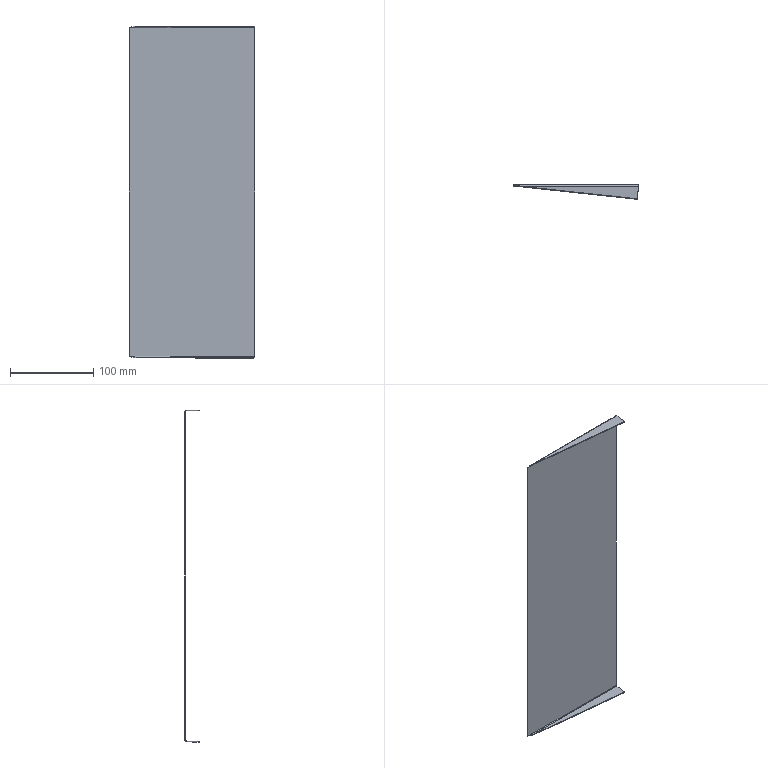Part | SolidWorks | features EdgeFlange 1, FlatPattern 1, MirrorPattern 1, SMBaseFlange 1, SheetMetal 1 | 1 solid | 20 faces | box 150.5 x 17 x 399 mm | volume 62251 mm3 | plane 12 | spline 4 | cylinder 4 | commonest cylinder face diameters 2 x2 4 x2
STEP:
#1=CARTESIAN_POINT('',(0.,-1.,-197.5));
#2=VERTEX_POINT('',#1);
#3=CARTESIAN_POINT('',(-150.5,-1.,-197.5));
#4=VERTEX_POINT('',#3);
#5=CARTESIAN_POINT('',(0.,-1.,-197.5));
#6=DIRECTION('',(-1.,0.,0.));
#7=VECTOR('',#6,1000.);
#8=LINE('',#5,#7);
#9=EDGE_CURVE('',#2,#4,#8,.T.);
#10=ORIENTED_EDGE('',*,*,#9,.F.);
#11=CARTESIAN_POINT('',(0.,-1.,197.5));
#12=VERTEX_POINT('',#11);
#13=CARTESIAN_POINT('',(0.,-1.,199.5));
#14=DIRECTION('',(0.,0.,-1.));
#15=VECTOR('',#14,1000.);
#16=LINE('',#13,#15);
#17=EDGE_CURVE('',#12,#2,#16,.T.);
#18=ORIENTED_EDGE('',*,*,#17,.F.);
#19=CARTESIAN_POINT('',(-150.5,-1.,197.5));
#20=VERTEX_POINT('',#19);
#21=CARTESIAN_POINT('',(-150.5,-1.,197.5));
#22=DIRECTION('',(1.,0.,0.));
#23=VECTOR('',#22,1000.);
#24=LINE('',#21,#23);
#25=EDGE_CURVE('',#20,#12,#24,.T.);
#26=ORIENTED_EDGE('',*,*,#25,.F.);
#27=CARTESIAN_POINT('',(-150.5,-1.,199.5));
#28=DIRECTION('',(0.,0.,-1.));
#29=VECTOR('',#28,1000.);
#30=LINE('',#27,#29);
#31=EDGE_CURVE('',#20,#4,#30,.T.);
#32=ORIENTED_EDGE('',*,*,#31,.T.);
#33=EDGE_LOOP('',(#10,#18,#26,#32));
#34=FACE_OUTER_BOUND('',#33,.T.);
#35=CARTESIAN_POINT('',(-150.5,-1.,199.5));
#36=DIRECTION('',(0.,1.,0.));
#37=DIRECTION('',(0.,0.,1.));
#38=AXIS2_PLACEMENT_3D('',#35,#36,#37);
#39=PLANE('',#38);
#40=ADVANCED_FACE('',(#34),#39,.F.);
#41=CARTESIAN_POINT('',(0.,0.,197.5));
#42=VERTEX_POINT('',#41);
#43=CARTESIAN_POINT('',(0.,0.,-197.5));
#44=VERTEX_POINT('',#43);
#45=CARTESIAN_POINT('',(0.,0.,199.5));
#46=DIRECTION('',(0.,0.,-1.));
#47=VECTOR('',#46,1000.);
#48=LINE('',#45,#47);
#49=EDGE_CURVE('',#42,#44,#48,.T.);
#50=ORIENTED_EDGE('',*,*,#49,.T.);
#51=CARTESIAN_POINT('',(-150.5,0.,-197.5));
#52=VERTEX_POINT('',#51);
#53=CARTESIAN_POINT('',(0.,0.,-197.5));
#54=DIRECTION('',(-1.,0.,0.));
#55=VECTOR('',#54,1000.);
#56=LINE('',#53,#55);
#57=EDGE_CURVE('',#44,#52,#56,.T.);
#58=ORIENTED_EDGE('',*,*,#57,.T.);
#59=CARTESIAN_POINT('',(-150.5,0.,197.5));
#60=VERTEX_POINT('',#59);
#61=CARTESIAN_POINT('',(-150.5,0.,199.5));
#62=DIRECTION('',(0.,0.,-1.));
#63=VECTOR('',#62,1000.);
#64=LINE('',#61,#63);
#65=EDGE_CURVE('',#60,#52,#64,.T.);
#66=ORIENTED_EDGE('',*,*,#65,.F.);
#67=CARTESIAN_POINT('',(-150.5,0.,197.5));
#68=DIRECTION('',(1.,0.,0.));
#69=VECTOR('',#68,1000.);
#70=LINE('',#67,#69);
#71=EDGE_CURVE('',#60,#42,#70,.T.);
#72=ORIENTED_EDGE('',*,*,#71,.T.);
#73=EDGE_LOOP('',(#50,#58,#66,#72));
#74=FACE_OUTER_BOUND('',#73,.T.);
#75=CARTESIAN_POINT('',(-150.5,0.,199.5));
#76=DIRECTION('',(0.,1.,0.));
#77=DIRECTION('',(0.,0.,1.));
#78=AXIS2_PLACEMENT_3D('',#75,#76,#77);
#79=PLANE('',#78);
#80=ADVANCED_FACE('',(#74),#79,.T.);
#81=ORIENTED_EDGE('',*,*,#17,.T.);
#82=CARTESIAN_POINT('',(0.,-1.,-197.5));
#83=DIRECTION('',(0.,1.,0.));
#84=VECTOR('',#83,1000.);
#85=LINE('',#82,#84);
#86=EDGE_CURVE('',#2,#44,#85,.T.);
#87=ORIENTED_EDGE('',*,*,#86,.T.);
#88=ORIENTED_EDGE('',*,*,#49,.F.);
#89=CARTESIAN_POINT('',(0.,-1.,197.5));
#90=DIRECTION('',(0.,1.,0.));
#91=VECTOR('',#90,1000.);
#92=LINE('',#89,#91);
#93=EDGE_CURVE('',#12,#42,#92,.T.);
#94=ORIENTED_EDGE('',*,*,#93,.F.);
#95=EDGE_LOOP('',(#81,#87,#88,#94));
#96=FACE_OUTER_BOUND('',#95,.T.);
#97=CARTESIAN_POINT('',(0.,0.,199.5));
#98=DIRECTION('',(1.,0.,0.));
#99=DIRECTION('',(0.,0.,-1.));
#100=AXIS2_PLACEMENT_3D('',#97,#98,#99);
#101=PLANE('',#100);
#102=ADVANCED_FACE('',(#96),#101,.T.);
#103=CARTESIAN_POINT('',(-150.5,-1.,-197.5));
#104=DIRECTION('',(0.,1.,0.));
#105=VECTOR('',#104,1000.);
#106=LINE('',#103,#105);
#107=EDGE_CURVE('',#4,#52,#106,.T.);
#108=ORIENTED_EDGE('',*,*,#107,.F.);
#109=ORIENTED_EDGE('',*,*,#31,.F.);
#110=CARTESIAN_POINT('',(-150.5,-1.,197.5));
#111=DIRECTION('',(0.,1.,0.));
#112=VECTOR('',#111,1000.);
#113=LINE('',#110,#112);
#114=EDGE_CURVE('',#20,#60,#113,.T.);
#115=ORIENTED_EDGE('',*,*,#114,.T.);
#116=ORIENTED_EDGE('',*,*,#65,.T.);
#117=EDGE_LOOP('',(#108,#109,#115,#116));
#118=FACE_OUTER_BOUND('',#117,.T.);
#119=CARTESIAN_POINT('',(-150.5,-1.,199.5));
#120=DIRECTION('',(-1.,0.,0.));
#121=DIRECTION('',(0.,0.,1.));
#122=AXIS2_PLACEMENT_3D('',#119,#120,#121);
#123=PLANE('',#122);
#124=ADVANCED_FACE('',(#118),#123,.T.);
#125=CARTESIAN_POINT('',(-0.1075,-2.,198.5));
#126=VERTEX_POINT('',#125);
#127=CARTESIAN_POINT('',(-0.1075,-2.,199.5));
#128=VERTEX_POINT('',#127);
#129=CARTESIAN_POINT('',(-0.1075,-2.,199.5));
#130=DIRECTION('',(0.,0.,1.));
#131=VECTOR('',#130,1000.);
#132=LINE('',#129,#131);
#133=EDGE_CURVE('',#126,#128,#132,.T.);
#134=ORIENTED_EDGE('',*,*,#133,.F.);
#135=CARTESIAN_POINT('',(0.,-1.,197.5));
#136=CARTESIAN_POINT('',(-0.01792,-1.,197.762));
#137=CARTESIAN_POINT('',(-0.03585,-1.108,198.022));
#138=CARTESIAN_POINT('',(-0.07169,-1.478,198.392));
#139=CARTESIAN_POINT('',(-0.08962,-1.738,198.5));
#140=CARTESIAN_POINT('',(-0.1075,-2.,198.5));
#141=B_SPLINE_CURVE_WITH_KNOTS('',3,(#135,#136,#137,#138,#139,#140),.UNSPECIFIED.,.F.,.F.,(4,2,4),(0.,0.5,1.),.UNSPECIFIED.);
#142=EDGE_CURVE('',#12,#126,#141,.T.);
#143=ORIENTED_EDGE('',*,*,#142,.F.);
#144=ORIENTED_EDGE('',*,*,#93,.T.);
#145=CARTESIAN_POINT('',(0.,0.,197.5));
#146=CARTESIAN_POINT('',(-0.008962,0.,197.762));
#147=CARTESIAN_POINT('',(-0.01792,-0.05205,198.023));
#148=CARTESIAN_POINT('',(-0.03585,-0.2524,198.507));
#149=CARTESIAN_POINT('',(-0.04481,-0.4007,198.729));
#150=CARTESIAN_POINT('',(-0.06273,-0.7709,199.099));
#151=CARTESIAN_POINT('',(-0.07169,-0.9928,199.248));
#152=CARTESIAN_POINT('',(-0.08962,-1.477,199.448));
#153=CARTESIAN_POINT('',(-0.09858,-1.738,199.5));
#154=CARTESIAN_POINT('',(-0.1075,-2.,199.5));
#155=B_SPLINE_CURVE_WITH_KNOTS('',3,(#145,#146,#147,#148,#149,#150,#151,#152,#153,#154),.UNSPECIFIED.,.F.,.F.,(4,2,2,2,4),(0.,0.25,0.5,0.75,1.),.UNSPECIFIED.);
#156=EDGE_CURVE('',#42,#128,#155,.T.);
#157=ORIENTED_EDGE('',*,*,#156,.T.);
#158=EDGE_LOOP('',(#134,#143,#144,#157));
#159=FACE_OUTER_BOUND('',#158,.T.);
#160=CARTESIAN_POINT('',(0.,0.01,197.5));
#161=CARTESIAN_POINT('',(-0.008963,0.01,197.763));
#162=CARTESIAN_POINT('',(-0.01792,-0.04231,198.026));
#163=CARTESIAN_POINT('',(-0.03585,-0.2437,198.512));
#164=CARTESIAN_POINT('',(-0.04481,-0.3927,198.735));
#165=CARTESIAN_POINT('',(-0.06273,-0.7648,199.107));
#166=CARTESIAN_POINT('',(-0.07169,-0.9877,199.256));
#167=CARTESIAN_POINT('',(-0.08962,-1.474,199.458));
#168=CARTESIAN_POINT('',(-0.09858,-1.737,199.51));
#169=CARTESIAN_POINT('',(-0.1075,-2.,199.51));
#170=CARTESIAN_POINT('',(0.,0.,197.5));
#171=CARTESIAN_POINT('',(-0.008963,0.,197.762));
#172=CARTESIAN_POINT('',(-0.01792,-0.05205,198.023));
#173=CARTESIAN_POINT('',(-0.03585,-0.2524,198.507));
#174=CARTESIAN_POINT('',(-0.04481,-0.4007,198.729));
#175=CARTESIAN_POINT('',(-0.06273,-0.7709,199.099));
#176=CARTESIAN_POINT('',(-0.07169,-0.9928,199.248));
#177=CARTESIAN_POINT('',(-0.08962,-1.477,199.448));
#178=CARTESIAN_POINT('',(-0.09858,-1.738,199.5));
#179=CARTESIAN_POINT('',(-0.1075,-2.,199.5));
#180=CARTESIAN_POINT('',(0.,-1.,197.5));
#181=CARTESIAN_POINT('',(-0.008963,-1.,197.631));
#182=CARTESIAN_POINT('',(-0.01792,-1.026,197.762));
#183=CARTESIAN_POINT('',(-0.03585,-1.126,198.004));
#184=CARTESIAN_POINT('',(-0.04481,-1.2,198.115));
#185=CARTESIAN_POINT('',(-0.06273,-1.385,198.3));
#186=CARTESIAN_POINT('',(-0.07169,-1.496,198.374));
#187=CARTESIAN_POINT('',(-0.08962,-1.738,198.474));
#188=CARTESIAN_POINT('',(-0.09858,-1.869,198.5));
#189=CARTESIAN_POINT('',(-0.1075,-2.,198.5));
#190=CARTESIAN_POINT('',(0.,-1.01,197.5));
#191=CARTESIAN_POINT('',(-0.008963,-1.01,197.63));
#192=CARTESIAN_POINT('',(-0.01792,-1.036,197.759));
#193=CARTESIAN_POINT('',(-0.03585,-1.135,197.999));
#194=CARTESIAN_POINT('',(-0.04481,-1.208,198.108));
#195=CARTESIAN_POINT('',(-0.06273,-1.392,198.292));
#196=CARTESIAN_POINT('',(-0.07169,-1.501,198.365));
#197=CARTESIAN_POINT('',(-0.08962,-1.741,198.464));
#198=CARTESIAN_POINT('',(-0.09858,-1.87,198.49));
#199=CARTESIAN_POINT('',(-0.1075,-2.,198.49));
#200=B_SPLINE_SURFACE_WITH_KNOTS('',1,3,((#160,#161,#162,#163,#164,#165,#166,#167,#168,#169),(#170,#171,#172,#173,#174,#175,#176,#177,#178,#179),(#180,#181,#182,#183,#184,#185,#186,#187,#188,#189),(#190,#191,#192,#193,#194,#195,#196,#197,#198,#199)),.UNSPECIFIED.,.F.,.F.,.F.,(2,1,1,2),(4,2,2,2,4),(-0.01,0.,1.,1.01),(0.,0.25,0.5,0.75,1.),.UNSPECIFIED.);
#201=ADVANCED_FACE('',(#159),#200,.F.);
#202=CARTESIAN_POINT('',(-141.201,-2.,198.5));
#203=VERTEX_POINT('',#202);
#204=CARTESIAN_POINT('',(-141.201,-2.,198.5));
#205=CARTESIAN_POINT('',(-141.977,-1.869,198.5));
#206=CARTESIAN_POINT('',(-142.752,-1.738,198.474));
#207=CARTESIAN_POINT('',(-144.302,-1.496,198.374));
#208=CARTESIAN_POINT('',(-145.076,-1.385,198.3));
#209=CARTESIAN_POINT('',(-146.626,-1.2,198.115));
#210=CARTESIAN_POINT('',(-147.401,-1.126,198.003));
#211=CARTESIAN_POINT('',(-148.95,-1.026,197.762));
#212=CARTESIAN_POINT('',(-149.725,-1.,197.631));
#213=CARTESIAN_POINT('',(-150.5,-1.,197.5));
#214=B_SPLINE_CURVE_WITH_KNOTS('',3,(#204,#205,#206,#207,#208,#209,#210,#211,#212,#213),.UNSPECIFIED.,.F.,.F.,(4,2,2,2,4),(0.,0.002358,0.004717,0.007075,0.009434),.UNSPECIFIED.);
#215=EDGE_CURVE('',#203,#20,#214,.T.);
#216=ORIENTED_EDGE('',*,*,#215,.F.);
#217=CARTESIAN_POINT('',(-141.201,-2.,199.5));
#218=VERTEX_POINT('',#217);
#219=CARTESIAN_POINT('',(-141.201,-2.,198.5));
#220=DIRECTION('',(0.,0.,1.));
#221=VECTOR('',#220,1000.);
#222=LINE('',#219,#221);
#223=EDGE_CURVE('',#203,#218,#222,.T.);
#224=ORIENTED_EDGE('',*,*,#223,.T.);
#225=CARTESIAN_POINT('',(-141.201,-2.,199.5));
#226=CARTESIAN_POINT('',(-141.978,-1.737,199.5));
#227=CARTESIAN_POINT('',(-142.755,-1.475,199.448));
#228=CARTESIAN_POINT('',(-144.307,-0.991,199.247));
#229=CARTESIAN_POINT('',(-145.08,-0.7698,199.099));
#230=CARTESIAN_POINT('',(-146.632,-0.3993,198.727));
#231=CARTESIAN_POINT('',(-147.407,-0.2515,198.505));
#232=CARTESIAN_POINT('',(-148.951,-0.05209,198.023));
#233=CARTESIAN_POINT('',(-149.723,0.,197.763));
#234=CARTESIAN_POINT('',(-150.5,0.,197.5));
#235=B_SPLINE_CURVE_WITH_KNOTS('',3,(#225,#226,#227,#228,#229,#230,#231,#232,#233,#234),.UNSPECIFIED.,.F.,.F.,(4,2,2,2,4),(0.,0.002458,0.004915,0.007373,0.009831),.UNSPECIFIED.);
#236=EDGE_CURVE('',#218,#60,#235,.T.);
#237=ORIENTED_EDGE('',*,*,#236,.T.);
#238=ORIENTED_EDGE('',*,*,#114,.F.);
#239=EDGE_LOOP('',(#216,#224,#237,#238));
#240=FACE_OUTER_BOUND('',#239,.T.);
#241=CARTESIAN_POINT('',(-141.201,-2.,199.51));
#242=CARTESIAN_POINT('',(-141.976,-1.737,199.51));
#243=CARTESIAN_POINT('',(-142.751,-1.474,199.458));
#244=CARTESIAN_POINT('',(-144.301,-0.9877,199.256));
#245=CARTESIAN_POINT('',(-145.076,-0.7648,199.107));
#246=CARTESIAN_POINT('',(-146.626,-0.3927,198.735));
#247=CARTESIAN_POINT('',(-147.4,-0.2437,198.512));
#248=CARTESIAN_POINT('',(-148.95,-0.04231,198.026));
#249=CARTESIAN_POINT('',(-149.725,0.01,197.763));
#250=CARTESIAN_POINT('',(-150.5,0.01,197.5));
#251=CARTESIAN_POINT('',(-141.201,-2.,199.5));
#252=CARTESIAN_POINT('',(-141.976,-1.738,199.5));
#253=CARTESIAN_POINT('',(-142.751,-1.477,199.448));
#254=CARTESIAN_POINT('',(-144.301,-0.9928,199.248));
#255=CARTESIAN_POINT('',(-145.076,-0.7709,199.099));
#256=CARTESIAN_POINT('',(-146.626,-0.4007,198.729));
#257=CARTESIAN_POINT('',(-147.4,-0.2524,198.507));
#258=CARTESIAN_POINT('',(-148.95,-0.05205,198.023));
#259=CARTESIAN_POINT('',(-149.725,0.,197.762));
#260=CARTESIAN_POINT('',(-150.5,0.,197.5));
#261=CARTESIAN_POINT('',(-141.201,-2.,198.5));
#262=CARTESIAN_POINT('',(-141.976,-1.869,198.5));
#263=CARTESIAN_POINT('',(-142.751,-1.738,198.474));
#264=CARTESIAN_POINT('',(-144.301,-1.496,198.374));
#265=CARTESIAN_POINT('',(-145.076,-1.385,198.3));
#266=CARTESIAN_POINT('',(-146.626,-1.2,198.115));
#267=CARTESIAN_POINT('',(-147.4,-1.126,198.004));
#268=CARTESIAN_POINT('',(-148.95,-1.026,197.762));
#269=CARTESIAN_POINT('',(-149.725,-1.,197.631));
#270=CARTESIAN_POINT('',(-150.5,-1.,197.5));
#271=CARTESIAN_POINT('',(-141.201,-2.,198.49));
#272=CARTESIAN_POINT('',(-141.976,-1.87,198.49));
#273=CARTESIAN_POINT('',(-142.751,-1.741,198.464));
#274=CARTESIAN_POINT('',(-144.301,-1.501,198.365));
#275=CARTESIAN_POINT('',(-145.076,-1.392,198.292));
#276=CARTESIAN_POINT('',(-146.626,-1.208,198.108));
#277=CARTESIAN_POINT('',(-147.4,-1.135,197.999));
#278=CARTESIAN_POINT('',(-148.95,-1.036,197.759));
#279=CARTESIAN_POINT('',(-149.725,-1.01,197.63));
#280=CARTESIAN_POINT('',(-150.5,-1.01,197.5));
#281=B_SPLINE_SURFACE_WITH_KNOTS('',1,3,((#241,#242,#243,#244,#245,#246,#247,#248,#249,#250),(#251,#252,#253,#254,#255,#256,#257,#258,#259,#260),(#261,#262,#263,#264,#265,#266,#267,#268,#269,#270),(#271,#272,#273,#274,#275,#276,#277,#278,#279,#280)),.UNSPECIFIED.,.F.,.F.,.F.,(2,1,1,2),(4,2,2,2,4),(-0.01,0.,1.,1.01),(0.,0.25,0.5,0.75,1.),.UNSPECIFIED.);
#282=ADVANCED_FACE('',(#240),#281,.F.);
#283=ORIENTED_EDGE('',*,*,#71,.F.);
#284=ORIENTED_EDGE('',*,*,#236,.F.);
#285=CARTESIAN_POINT('',(-0.1075,-2.,199.5));
#286=DIRECTION('',(1.,0.,0.));
#287=VECTOR('',#286,1000.);
#288=LINE('',#285,#287);
#289=EDGE_CURVE('',#218,#128,#288,.T.);
#290=ORIENTED_EDGE('',*,*,#289,.T.);
#291=ORIENTED_EDGE('',*,*,#156,.F.);
#292=EDGE_LOOP('',(#283,#284,#290,#291));
#293=FACE_OUTER_BOUND('',#292,.T.);
#294=CARTESIAN_POINT('',(-150.5,-2.,197.5));
#295=DIRECTION('',(-1.,0.,0.));
#296=DIRECTION('',(0.,0.,1.));
#297=AXIS2_PLACEMENT_3D('',#294,#295,#296);
#298=CYLINDRICAL_SURFACE('',#297,2.);
#299=ADVANCED_FACE('',(#293),#298,.T.);
#300=ORIENTED_EDGE('',*,*,#25,.T.);
#301=ORIENTED_EDGE('',*,*,#142,.T.);
#302=CARTESIAN_POINT('',(-0.1075,-2.,198.5));
#303=DIRECTION('',(-1.,0.,0.));
#304=VECTOR('',#303,1000.);
#305=LINE('',#302,#304);
#306=EDGE_CURVE('',#126,#203,#305,.T.);
#307=ORIENTED_EDGE('',*,*,#306,.T.);
#308=ORIENTED_EDGE('',*,*,#215,.T.);
#309=EDGE_LOOP('',(#300,#301,#307,#308));
#310=FACE_OUTER_BOUND('',#309,.T.);
#311=CARTESIAN_POINT('',(-150.5,-2.,197.5));
#312=DIRECTION('',(-1.,0.,0.));
#313=DIRECTION('',(0.,0.,1.));
#314=AXIS2_PLACEMENT_3D('',#311,#312,#313);
#315=CYLINDRICAL_SURFACE('',#314,1.);
#316=ADVANCED_FACE('',(#310),#315,.F.);
#317=CARTESIAN_POINT('',(-1.721,-17.,199.5));
#318=VERTEX_POINT('',#317);
#319=CARTESIAN_POINT('',(-150.5,-1.,199.5));
#320=DIRECTION('',(-0.9943,0.1069,0.));
#321=VECTOR('',#320,1000.);
#322=LINE('',#319,#321);
#323=EDGE_CURVE('',#318,#218,#322,.T.);
#324=ORIENTED_EDGE('',*,*,#323,.T.);
#325=ORIENTED_EDGE('',*,*,#223,.F.);
#326=CARTESIAN_POINT('',(-1.721,-17.,198.5));
#327=VERTEX_POINT('',#326);
#328=CARTESIAN_POINT('',(-1.827,-16.989,198.5));
#329=DIRECTION('',(-0.9943,0.1069,0.));
#330=VECTOR('',#329,1000.);
#331=LINE('',#328,#330);
#332=EDGE_CURVE('',#327,#203,#331,.T.);
#333=ORIENTED_EDGE('',*,*,#332,.F.);
#334=CARTESIAN_POINT('',(-1.721,-17.,199.5));
#335=DIRECTION('',(0.,0.,-1.));
#336=VECTOR('',#335,1000.);
#337=LINE('',#334,#336);
#338=EDGE_CURVE('',#318,#327,#337,.T.);
#339=ORIENTED_EDGE('',*,*,#338,.F.);
#340=EDGE_LOOP('',(#324,#325,#333,#339));
#341=FACE_OUTER_BOUND('',#340,.T.);
#342=CARTESIAN_POINT('',(-150.5,-1.,199.5));
#343=DIRECTION('',(-0.1069,-0.9943,0.));
#344=DIRECTION('',(0.9943,-0.1069,0.));
#345=AXIS2_PLACEMENT_3D('',#342,#343,#344);
#346=PLANE('',#345);
#347=ADVANCED_FACE('',(#341),#346,.T.);
#348=CARTESIAN_POINT('',(0.1063,-0.01143,198.5));
#349=DIRECTION('',(-0.1069,-0.9943,0.));
#350=VECTOR('',#349,1000.);
#351=LINE('',#348,#350);
#352=EDGE_CURVE('',#126,#327,#351,.T.);
#353=ORIENTED_EDGE('',*,*,#352,.F.);
#354=ORIENTED_EDGE('',*,*,#133,.T.);
#355=CARTESIAN_POINT('',(-1.721,-17.,199.5));
#356=DIRECTION('',(-0.1069,-0.9943,0.));
#357=VECTOR('',#356,1000.);
#358=LINE('',#355,#357);
#359=EDGE_CURVE('',#128,#318,#358,.T.);
#360=ORIENTED_EDGE('',*,*,#359,.T.);
#361=ORIENTED_EDGE('',*,*,#338,.T.);
#362=EDGE_LOOP('',(#353,#354,#360,#361));
#363=FACE_OUTER_BOUND('',#362,.T.);
#364=CARTESIAN_POINT('',(-1.721,-17.,199.5));
#365=DIRECTION('',(0.9943,-0.1069,0.));
#366=DIRECTION('',(0.1069,0.9943,0.));
#367=AXIS2_PLACEMENT_3D('',#364,#365,#366);
#368=PLANE('',#367);
#369=ADVANCED_FACE('',(#363),#368,.T.);
#370=ORIENTED_EDGE('',*,*,#289,.F.);
#371=ORIENTED_EDGE('',*,*,#323,.F.);
#372=ORIENTED_EDGE('',*,*,#359,.F.);
#373=EDGE_LOOP('',(#370,#371,#372));
#374=FACE_OUTER_BOUND('',#373,.T.);
#375=CARTESIAN_POINT('',(0.,0.,199.5));
#376=DIRECTION('',(0.,0.,-1.));
#377=DIRECTION('',(0.,1.,0.));
#378=AXIS2_PLACEMENT_3D('',#375,#376,#377);
#379=PLANE('',#378);
#380=ADVANCED_FACE('',(#374),#379,.F.);
#381=ORIENTED_EDGE('',*,*,#332,.T.);
#382=ORIENTED_EDGE('',*,*,#306,.F.);
#383=ORIENTED_EDGE('',*,*,#352,.T.);
#384=EDGE_LOOP('',(#381,#382,#383));
#385=FACE_OUTER_BOUND('',#384,.T.);
#386=CARTESIAN_POINT('',(0.,0.,198.5));
#387=DIRECTION('',(0.,0.,-1.));
#388=DIRECTION('',(0.,1.,0.));
#389=AXIS2_PLACEMENT_3D('',#386,#387,#388);
#390=PLANE('',#389);
#391=ADVANCED_FACE('',(#385),#390,.T.);
#392=CARTESIAN_POINT('',(-141.201,-2.,-198.5));
#393=VERTEX_POINT('',#392);
#394=CARTESIAN_POINT('',(-141.201,-2.,-199.5));
#395=VERTEX_POINT('',#394);
#396=CARTESIAN_POINT('',(-141.201,-2.,-199.5));
#397=DIRECTION('',(0.,0.,-1.));
#398=VECTOR('',#397,1000.);
#399=LINE('',#396,#398);
#400=EDGE_CURVE('',#393,#395,#399,.T.);
#401=ORIENTED_EDGE('',*,*,#400,.F.);
#402=CARTESIAN_POINT('',(-150.5,-1.,-197.5));
#403=CARTESIAN_POINT('',(-149.725,-1.,-197.631));
#404=CARTESIAN_POINT('',(-148.949,-1.026,-197.762));
#405=CARTESIAN_POINT('',(-147.399,-1.126,-198.004));
#406=CARTESIAN_POINT('',(-146.625,-1.2,-198.115));
#407=CARTESIAN_POINT('',(-145.076,-1.385,-198.3));
#408=CARTESIAN_POINT('',(-144.3,-1.497,-198.374));
#409=CARTESIAN_POINT('',(-142.751,-1.738,-198.474));
#410=CARTESIAN_POINT('',(-141.977,-1.869,-198.5));
#411=CARTESIAN_POINT('',(-141.201,-2.,-198.5));
#412=B_SPLINE_CURVE_WITH_KNOTS('',3,(#402,#403,#404,#405,#406,#407,#408,#409,#410,#411),.UNSPECIFIED.,.F.,.F.,(4,2,2,2,4),(0.,0.002358,0.004717,0.007075,0.009434),.UNSPECIFIED.);
#413=EDGE_CURVE('',#4,#393,#412,.T.);
#414=ORIENTED_EDGE('',*,*,#413,.F.);
#415=ORIENTED_EDGE('',*,*,#107,.T.);
#416=CARTESIAN_POINT('',(-150.5,0.,-197.5));
#417=CARTESIAN_POINT('',(-149.723,0.,-197.763));
#418=CARTESIAN_POINT('',(-148.946,-0.05235,-198.025));
#419=CARTESIAN_POINT('',(-147.395,-0.2534,-198.509));
#420=CARTESIAN_POINT('',(-146.622,-0.4014,-198.73));
#421=CARTESIAN_POINT('',(-145.069,-0.7726,-199.101));
#422=CARTESIAN_POINT('',(-144.295,-0.9947,-199.249));
#423=CARTESIAN_POINT('',(-142.75,-1.477,-199.448));
#424=CARTESIAN_POINT('',(-141.978,-1.737,-199.5));
#425=CARTESIAN_POINT('',(-141.201,-2.,-199.5));
#426=B_SPLINE_CURVE_WITH_KNOTS('',3,(#416,#417,#418,#419,#420,#421,#422,#423,#424,#425),.UNSPECIFIED.,.F.,.F.,(4,2,2,2,4),(0.,0.002458,0.004915,0.007373,0.009831),.UNSPECIFIED.);
#427=EDGE_CURVE('',#52,#395,#426,.T.);
#428=ORIENTED_EDGE('',*,*,#427,.T.);
#429=EDGE_LOOP('',(#401,#414,#415,#428));
#430=FACE_OUTER_BOUND('',#429,.T.);
#431=CARTESIAN_POINT('',(-150.5,0.01,-197.5));
#432=CARTESIAN_POINT('',(-149.725,0.01,-197.763));
#433=CARTESIAN_POINT('',(-148.95,-0.04231,-198.026));
#434=CARTESIAN_POINT('',(-147.4,-0.2437,-198.512));
#435=CARTESIAN_POINT('',(-146.626,-0.3927,-198.735));
#436=CARTESIAN_POINT('',(-145.076,-0.7648,-199.107));
#437=CARTESIAN_POINT('',(-144.301,-0.9877,-199.256));
#438=CARTESIAN_POINT('',(-142.751,-1.474,-199.458));
#439=CARTESIAN_POINT('',(-141.976,-1.737,-199.51));
#440=CARTESIAN_POINT('',(-141.201,-2.,-199.51));
#441=CARTESIAN_POINT('',(-150.5,0.,-197.5));
#442=CARTESIAN_POINT('',(-149.725,0.,-197.762));
#443=CARTESIAN_POINT('',(-148.95,-0.05205,-198.023));
#444=CARTESIAN_POINT('',(-147.4,-0.2524,-198.507));
#445=CARTESIAN_POINT('',(-146.626,-0.4007,-198.729));
#446=CARTESIAN_POINT('',(-145.076,-0.7709,-199.099));
#447=CARTESIAN_POINT('',(-144.301,-0.9928,-199.248));
#448=CARTESIAN_POINT('',(-142.751,-1.477,-199.448));
#449=CARTESIAN_POINT('',(-141.976,-1.738,-199.5));
#450=CARTESIAN_POINT('',(-141.201,-2.,-199.5));
#451=CARTESIAN_POINT('',(-150.5,-1.,-197.5));
#452=CARTESIAN_POINT('',(-149.725,-1.,-197.631));
#453=CARTESIAN_POINT('',(-148.95,-1.026,-197.762));
#454=CARTESIAN_POINT('',(-147.4,-1.126,-198.004));
#455=CARTESIAN_POINT('',(-146.626,-1.2,-198.115));
#456=CARTESIAN_POINT('',(-145.076,-1.385,-198.3));
#457=CARTESIAN_POINT('',(-144.301,-1.496,-198.374));
#458=CARTESIAN_POINT('',(-142.751,-1.738,-198.474));
#459=CARTESIAN_POINT('',(-141.976,-1.869,-198.5));
#460=CARTESIAN_POINT('',(-141.201,-2.,-198.5));
#461=CARTESIAN_POINT('',(-150.5,-1.01,-197.5));
#462=CARTESIAN_POINT('',(-149.725,-1.01,-197.63));
#463=CARTESIAN_POINT('',(-148.95,-1.036,-197.759));
#464=CARTESIAN_POINT('',(-147.4,-1.135,-197.999));
#465=CARTESIAN_POINT('',(-146.626,-1.208,-198.108));
#466=CARTESIAN_POINT('',(-145.076,-1.392,-198.292));
#467=CARTESIAN_POINT('',(-144.301,-1.501,-198.365));
#468=CARTESIAN_POINT('',(-142.751,-1.741,-198.464));
#469=CARTESIAN_POINT('',(-141.976,-1.87,-198.49));
#470=CARTESIAN_POINT('',(-141.201,-2.,-198.49));
#471=B_SPLINE_SURFACE_WITH_KNOTS('',1,3,((#431,#432,#433,#434,#435,#436,#437,#438,#439,#440),(#441,#442,#443,#444,#445,#446,#447,#448,#449,#450),(#451,#452,#453,#454,#455,#456,#457,#458,#459,#460),(#461,#462,#463,#464,#465,#466,#467,#468,#469,#470)),.UNSPECIFIED.,.F.,.F.,.F.,(2,1,1,2),(4,2,2,2,4),(-0.01,0.,1.,1.01),(0.,0.25,0.5,0.75,1.),.UNSPECIFIED.);
#472=ADVANCED_FACE('',(#430),#471,.F.);
#473=CARTESIAN_POINT('',(-0.1075,-2.,-198.5));
#474=VERTEX_POINT('',#473);
#475=CARTESIAN_POINT('',(-0.1075,-2.,-198.5));
#476=CARTESIAN_POINT('',(-0.08962,-1.738,-198.5));
#477=CARTESIAN_POINT('',(-0.07169,-1.478,-198.392));
#478=CARTESIAN_POINT('',(-0.03585,-1.108,-198.022));
#479=CARTESIAN_POINT('',(-0.01792,-1.,-197.762));
#480=CARTESIAN_POINT('',(0.,-1.,-197.5));
#481=B_SPLINE_CURVE_WITH_KNOTS('',3,(#475,#476,#477,#478,#479,#480),.UNSPECIFIED.,.F.,.F.,(4,2,4),(0.,0.5,1.),.UNSPECIFIED.);
#482=EDGE_CURVE('',#474,#2,#481,.T.);
#483=ORIENTED_EDGE('',*,*,#482,.F.);
#484=CARTESIAN_POINT('',(-0.1075,-2.,-199.5));
#485=VERTEX_POINT('',#484);
#486=CARTESIAN_POINT('',(-0.1075,-2.,-198.5));
#487=DIRECTION('',(0.,0.,-1.));
#488=VECTOR('',#487,1000.);
#489=LINE('',#486,#488);
#490=EDGE_CURVE('',#474,#485,#489,.T.);
#491=ORIENTED_EDGE('',*,*,#490,.T.);
#492=CARTESIAN_POINT('',(-0.1075,-2.,-199.5));
#493=CARTESIAN_POINT('',(-0.09858,-1.738,-199.5));
#494=CARTESIAN_POINT('',(-0.08962,-1.477,-199.448));
#495=CARTESIAN_POINT('',(-0.07169,-0.9928,-199.248));
#496=CARTESIAN_POINT('',(-0.06273,-0.7709,-199.099));
#497=CARTESIAN_POINT('',(-0.04481,-0.4007,-198.729));
#498=CARTESIAN_POINT('',(-0.03585,-0.2524,-198.507));
#499=CARTESIAN_POINT('',(-0.01792,-0.05205,-198.023));
#500=CARTESIAN_POINT('',(-0.008962,0.,-197.762));
#501=CARTESIAN_POINT('',(0.,0.,-197.5));
#502=B_SPLINE_CURVE_WITH_KNOTS('',3,(#492,#493,#494,#495,#496,#497,#498,#499,#500,#501),.UNSPECIFIED.,.F.,.F.,(4,2,2,2,4),(0.,0.25,0.5,0.75,1.),.UNSPECIFIED.);
#503=EDGE_CURVE('',#485,#44,#502,.T.);
#504=ORIENTED_EDGE('',*,*,#503,.T.);
#505=ORIENTED_EDGE('',*,*,#86,.F.);
#506=EDGE_LOOP('',(#483,#491,#504,#505));
#507=FACE_OUTER_BOUND('',#506,.T.);
#508=CARTESIAN_POINT('',(-0.1075,-2.,-199.51));
#509=CARTESIAN_POINT('',(-0.09858,-1.737,-199.51));
#510=CARTESIAN_POINT('',(-0.08962,-1.474,-199.458));
#511=CARTESIAN_POINT('',(-0.07169,-0.9877,-199.256));
#512=CARTESIAN_POINT('',(-0.06273,-0.7648,-199.107));
#513=CARTESIAN_POINT('',(-0.04481,-0.3927,-198.735));
#514=CARTESIAN_POINT('',(-0.03585,-0.2437,-198.512));
#515=CARTESIAN_POINT('',(-0.01792,-0.04231,-198.026));
#516=CARTESIAN_POINT('',(-0.008963,0.01,-197.763));
#517=CARTESIAN_POINT('',(0.,0.01,-197.5));
#518=CARTESIAN_POINT('',(-0.1075,-2.,-199.5));
#519=CARTESIAN_POINT('',(-0.09858,-1.738,-199.5));
#520=CARTESIAN_POINT('',(-0.08962,-1.477,-199.448));
#521=CARTESIAN_POINT('',(-0.07169,-0.9928,-199.248));
#522=CARTESIAN_POINT('',(-0.06273,-0.7709,-199.099));
#523=CARTESIAN_POINT('',(-0.04481,-0.4007,-198.729));
#524=CARTESIAN_POINT('',(-0.03585,-0.2524,-198.507));
#525=CARTESIAN_POINT('',(-0.01792,-0.05205,-198.023));
#526=CARTESIAN_POINT('',(-0.008963,0.,-197.762));
#527=CARTESIAN_POINT('',(0.,0.,-197.5));
#528=CARTESIAN_POINT('',(-0.1075,-2.,-198.5));
#529=CARTESIAN_POINT('',(-0.09858,-1.869,-198.5));
#530=CARTESIAN_POINT('',(-0.08962,-1.738,-198.474));
#531=CARTESIAN_POINT('',(-0.07169,-1.496,-198.374));
#532=CARTESIAN_POINT('',(-0.06273,-1.385,-198.3));
#533=CARTESIAN_POINT('',(-0.04481,-1.2,-198.115));
#534=CARTESIAN_POINT('',(-0.03585,-1.126,-198.004));
#535=CARTESIAN_POINT('',(-0.01792,-1.026,-197.762));
#536=CARTESIAN_POINT('',(-0.008963,-1.,-197.631));
#537=CARTESIAN_POINT('',(0.,-1.,-197.5));
#538=CARTESIAN_POINT('',(-0.1075,-2.,-198.49));
#539=CARTESIAN_POINT('',(-0.09858,-1.87,-198.49));
#540=CARTESIAN_POINT('',(-0.08962,-1.741,-198.464));
#541=CARTESIAN_POINT('',(-0.07169,-1.501,-198.365));
#542=CARTESIAN_POINT('',(-0.06273,-1.392,-198.292));
#543=CARTESIAN_POINT('',(-0.04481,-1.208,-198.108));
#544=CARTESIAN_POINT('',(-0.03585,-1.135,-197.999));
#545=CARTESIAN_POINT('',(-0.01792,-1.036,-197.759));
#546=CARTESIAN_POINT('',(-0.008963,-1.01,-197.63));
#547=CARTESIAN_POINT('',(0.,-1.01,-197.5));
#548=B_SPLINE_SURFACE_WITH_KNOTS('',1,3,((#508,#509,#510,#511,#512,#513,#514,#515,#516,#517),(#518,#519,#520,#521,#522,#523,#524,#525,#526,#527),(#528,#529,#530,#531,#532,#533,#534,#535,#536,#537),(#538,#539,#540,#541,#542,#543,#544,#545,#546,#547)),.UNSPECIFIED.,.F.,.F.,.F.,(2,1,1,2),(4,2,2,2,4),(-0.01,0.,1.,1.01),(0.,0.25,0.5,0.75,1.),.UNSPECIFIED.);
#549=ADVANCED_FACE('',(#507),#548,.F.);
#550=ORIENTED_EDGE('',*,*,#57,.F.);
#551=ORIENTED_EDGE('',*,*,#503,.F.);
#552=CARTESIAN_POINT('',(-141.201,-2.,-199.5));
#553=DIRECTION('',(-1.,0.,0.));
#554=VECTOR('',#553,1000.);
#555=LINE('',#552,#554);
#556=EDGE_CURVE('',#485,#395,#555,.T.);
#557=ORIENTED_EDGE('',*,*,#556,.T.);
#558=ORIENTED_EDGE('',*,*,#427,.F.);
#559=EDGE_LOOP('',(#550,#551,#557,#558));
#560=FACE_OUTER_BOUND('',#559,.T.);
#561=CARTESIAN_POINT('',(0.,-2.,-197.5));
#562=DIRECTION('',(1.,0.,0.));
#563=DIRECTION('',(0.,0.,-1.));
#564=AXIS2_PLACEMENT_3D('',#561,#562,#563);
#565=CYLINDRICAL_SURFACE('',#564,2.);
#566=ADVANCED_FACE('',(#560),#565,.T.);
#567=ORIENTED_EDGE('',*,*,#9,.T.);
#568=ORIENTED_EDGE('',*,*,#413,.T.);
#569=CARTESIAN_POINT('',(-141.201,-2.,-198.5));
#570=DIRECTION('',(1.,0.,0.));
#571=VECTOR('',#570,1000.);
#572=LINE('',#569,#571);
#573=EDGE_CURVE('',#393,#474,#572,.T.);
#574=ORIENTED_EDGE('',*,*,#573,.T.);
#575=ORIENTED_EDGE('',*,*,#482,.T.);
#576=EDGE_LOOP('',(#567,#568,#574,#575));
#577=FACE_OUTER_BOUND('',#576,.T.);
#578=CARTESIAN_POINT('',(0.,-2.,-197.5));
#579=DIRECTION('',(1.,0.,0.));
#580=DIRECTION('',(0.,0.,-1.));
#581=AXIS2_PLACEMENT_3D('',#578,#579,#580);
#582=CYLINDRICAL_SURFACE('',#581,1.);
#583=ADVANCED_FACE('',(#577),#582,.F.);
#584=ORIENTED_EDGE('',*,*,#490,.F.);
#585=CARTESIAN_POINT('',(-1.721,-17.,-198.5));
#586=VERTEX_POINT('',#585);
#587=CARTESIAN_POINT('',(-1.721,-17.,-198.5));
#588=DIRECTION('',(-0.1069,-0.9943,0.));
#589=VECTOR('',#588,1000.);
#590=LINE('',#587,#589);
#591=EDGE_CURVE('',#474,#586,#590,.T.);
#592=ORIENTED_EDGE('',*,*,#591,.T.);
#593=CARTESIAN_POINT('',(-1.721,-17.,-199.5));
#594=VERTEX_POINT('',#593);
#595=CARTESIAN_POINT('',(-1.721,-17.,-199.5));
#596=DIRECTION('',(0.,0.,1.));
#597=VECTOR('',#596,1000.);
#598=LINE('',#595,#597);
#599=EDGE_CURVE('',#594,#586,#598,.T.);
#600=ORIENTED_EDGE('',*,*,#599,.F.);
#601=CARTESIAN_POINT('',(0.1063,-0.01143,-199.5));
#602=DIRECTION('',(-0.1069,-0.9943,0.));
#603=VECTOR('',#602,1000.);
#604=LINE('',#601,#603);
#605=EDGE_CURVE('',#485,#594,#604,.T.);
#606=ORIENTED_EDGE('',*,*,#605,.F.);
#607=EDGE_LOOP('',(#584,#592,#600,#606));
#608=FACE_OUTER_BOUND('',#607,.T.);
#609=CARTESIAN_POINT('',(-1.721,-17.,-199.5));
#610=DIRECTION('',(-0.9943,0.1069,0.));
#611=DIRECTION('',(-0.1069,-0.9943,0.));
#612=AXIS2_PLACEMENT_3D('',#609,#610,#611);
#613=PLANE('',#612);
#614=ADVANCED_FACE('',(#608),#613,.F.);
#615=ORIENTED_EDGE('',*,*,#400,.T.);
#616=CARTESIAN_POINT('',(-1.827,-16.989,-199.5));
#617=DIRECTION('',(-0.9943,0.1069,0.));
#618=VECTOR('',#617,1000.);
#619=LINE('',#616,#618);
#620=EDGE_CURVE('',#594,#395,#619,.T.);
#621=ORIENTED_EDGE('',*,*,#620,.F.);
#622=ORIENTED_EDGE('',*,*,#599,.T.);
#623=CARTESIAN_POINT('',(-150.5,-1.,-198.5));
#624=DIRECTION('',(-0.9943,0.1069,0.));
#625=VECTOR('',#624,1000.);
#626=LINE('',#623,#625);
#627=EDGE_CURVE('',#586,#393,#626,.T.);
#628=ORIENTED_EDGE('',*,*,#627,.T.);
#629=EDGE_LOOP('',(#615,#621,#622,#628));
#630=FACE_OUTER_BOUND('',#629,.T.);
#631=CARTESIAN_POINT('',(-150.5,-1.,-199.5));
#632=DIRECTION('',(0.1069,0.9943,0.));
#633=DIRECTION('',(-0.9943,0.1069,0.));
#634=AXIS2_PLACEMENT_3D('',#631,#632,#633);
#635=PLANE('',#634);
#636=ADVANCED_FACE('',(#630),#635,.F.);
#637=ORIENTED_EDGE('',*,*,#556,.F.);
#638=ORIENTED_EDGE('',*,*,#605,.T.);
#639=ORIENTED_EDGE('',*,*,#620,.T.);
#640=EDGE_LOOP('',(#637,#638,#639));
#641=FACE_OUTER_BOUND('',#640,.T.);
#642=CARTESIAN_POINT('',(0.,0.,-199.5));
#643=DIRECTION('',(0.,0.,1.));
#644=DIRECTION('',(0.,1.,0.));
#645=AXIS2_PLACEMENT_3D('',#642,#643,#644);
#646=PLANE('',#645);
#647=ADVANCED_FACE('',(#641),#646,.F.);
#648=ORIENTED_EDGE('',*,*,#591,.F.);
#649=ORIENTED_EDGE('',*,*,#573,.F.);
#650=ORIENTED_EDGE('',*,*,#627,.F.);
#651=EDGE_LOOP('',(#648,#649,#650));
#652=FACE_OUTER_BOUND('',#651,.T.);
#653=CARTESIAN_POINT('',(0.,0.,-198.5));
#654=DIRECTION('',(0.,0.,1.));
#655=DIRECTION('',(0.,1.,0.));
#656=AXIS2_PLACEMENT_3D('',#653,#654,#655);
#657=PLANE('',#656);
#658=ADVANCED_FACE('',(#652),#657,.T.);
#659=CLOSED_SHELL('',(#40,#80,#102,#124,#201,#282,#299,#316,#347,#369,#380,#391,#472,#549,#566,#583,#614,#636,#647,#658));
#660=MANIFOLD_SOLID_BREP('',#659);
#661=CARTESIAN_POINT('',(0.,0.,0.));
#662=DIRECTION('',(0.,0.,1.));
#663=DIRECTION('',(1.,0.,0.));
#664=AXIS2_PLACEMENT_3D('',#661,#662,#663);
#665=(LENGTH_UNIT()NAMED_UNIT(*)SI_UNIT(.MILLI.,.METRE.));
#666=UNCERTAINTY_MEASURE_WITH_UNIT(LENGTH_MEASURE(0.00001),#665,'','');
#667=(NAMED_UNIT(*)PLANE_ANGLE_UNIT()SI_UNIT($,.RADIAN.));
#668=(NAMED_UNIT(*)SI_UNIT($,.STERADIAN.)SOLID_ANGLE_UNIT());
#669=(GEOMETRIC_REPRESENTATION_CONTEXT(3)GLOBAL_UNCERTAINTY_ASSIGNED_CONTEXT((#666))GLOBAL_UNIT_ASSIGNED_CONTEXT((#665,#667,#668))REPRESENTATION_CONTEXT('',''));
#670=ADVANCED_BREP_SHAPE_REPRESENTATION('',(#660,#664),#669);